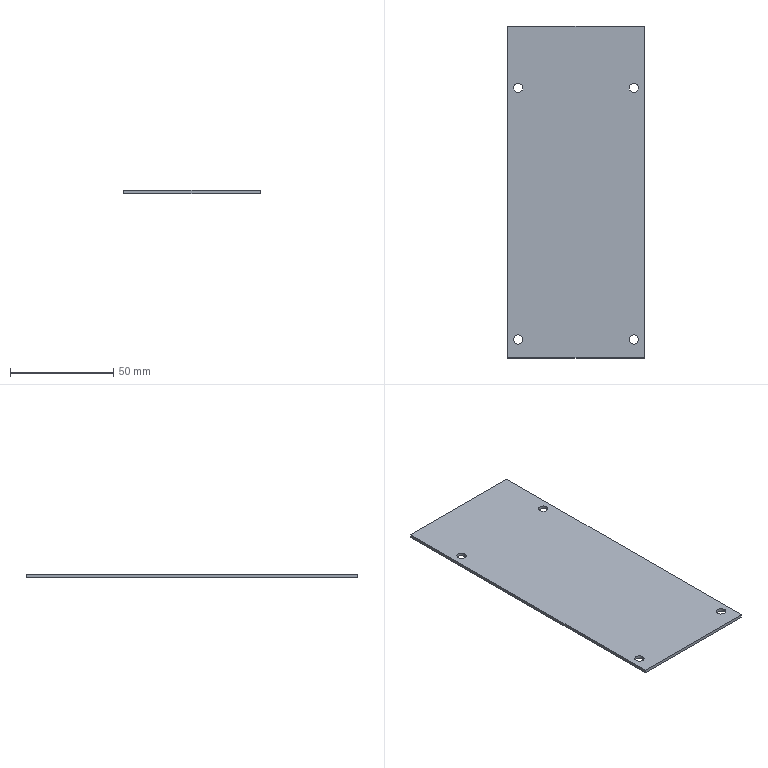Part | STEP file | 0245_219_Cover | 1 solid | 14 faces | box 66 x 161 x 1.5 mm | volume 15844 mm3 | cylinder 8 | plane 6 | commonest cylinder face diameters 4.5 x8
STEP:
#1=CARTESIAN_POINT('',(0.,0.,0.));
#2=DIRECTION('',(0.,0.,1.));
#3=DIRECTION('',(1.,0.,0.));
#4=AXIS2_PLACEMENT_3D('',#1,#2,#3);
#5=CARTESIAN_POINT('',(30.25,131.,0.));
#6=VERTEX_POINT('',#5);
#7=CARTESIAN_POINT('',(30.25,131.,1.5));
#8=VERTEX_POINT('',#7);
#9=CARTESIAN_POINT('',(30.25,131.,1.5));
#10=DIRECTION('',(0.,0.,1.));
#11=VECTOR('',#10,1.);
#12=LINE('',#9,#11);
#13=CARTESIAN_POINT('',(28.,131.,1.5));
#14=DIRECTION('',(0.,0.,1.));
#15=DIRECTION('',(1.,0.,0.));
#16=AXIS2_PLACEMENT_3D('',#13,#14,#15);
#17=CYLINDRICAL_SURFACE('',#16,2.25);
#18=CARTESIAN_POINT('',(6.283,0.));
#19=DIRECTION('',(0.,1.));
#20=VECTOR('',#19,1.);
#21=LINE('',#18,#20);
#22=(GEOMETRIC_REPRESENTATION_CONTEXT(2)PARAMETRIC_REPRESENTATION_CONTEXT()REPRESENTATION_CONTEXT('',''));
#23=DEFINITIONAL_REPRESENTATION('',(#21),#22);
#24=PCURVE('',#17,#23);
#25=CARTESIAN_POINT('',(28.,131.,1.5));
#26=DIRECTION('',(0.,0.,1.));
#27=DIRECTION('',(1.,0.,0.));
#28=AXIS2_PLACEMENT_3D('',#25,#26,#27);
#29=CYLINDRICAL_SURFACE('',#28,2.25);
#30=CARTESIAN_POINT('',(0.,0.));
#31=DIRECTION('',(0.,1.));
#32=VECTOR('',#31,1.);
#33=LINE('',#30,#32);
#34=(GEOMETRIC_REPRESENTATION_CONTEXT(2)PARAMETRIC_REPRESENTATION_CONTEXT()REPRESENTATION_CONTEXT('',''));
#35=DEFINITIONAL_REPRESENTATION('',(#33),#34);
#36=PCURVE('',#29,#35);
#37=SURFACE_CURVE('',#12,(#24,#36),.PCURVE_S1.);
#38=EDGE_CURVE('',#6,#8,#37,.T.);
#39=ORIENTED_EDGE('',*,*,#38,.T.);
#40=CARTESIAN_POINT('',(25.75,131.,1.5));
#41=VERTEX_POINT('',#40);
#42=CARTESIAN_POINT('',(28.,131.,1.5));
#43=DIRECTION('',(0.,0.,1.));
#44=DIRECTION('',(1.,0.,0.));
#45=AXIS2_PLACEMENT_3D('',#42,#43,#44);
#46=CIRCLE('',#45,2.25);
#47=CARTESIAN_POINT('',(0.,0.));
#48=DIRECTION('',(1.,0.));
#49=VECTOR('',#48,1.);
#50=LINE('',#47,#49);
#51=(GEOMETRIC_REPRESENTATION_CONTEXT(2)PARAMETRIC_REPRESENTATION_CONTEXT()REPRESENTATION_CONTEXT('',''));
#52=DEFINITIONAL_REPRESENTATION('',(#50),#51);
#53=PCURVE('',#17,#52);
#54=CARTESIAN_POINT('',(-33.,161.,1.5));
#55=DIRECTION('',(0.,0.,-1.));
#56=DIRECTION('',(-1.,0.,0.));
#57=AXIS2_PLACEMENT_3D('',#54,#55,#56);
#58=PLANE('',#57);
#59=CARTESIAN_POINT('',(-63.25,-30.));
#60=CARTESIAN_POINT('',(-63.25,-26.103));
#61=CARTESIAN_POINT('',(-59.875,-28.051));
#62=CARTESIAN_POINT('',(-56.5,-30.));
#63=CARTESIAN_POINT('',(-59.875,-31.949));
#64=CARTESIAN_POINT('',(-63.25,-33.897));
#65=CARTESIAN_POINT('',(-63.25,-30.));
#66=(BOUNDED_CURVE()B_SPLINE_CURVE(2,(#59,#60,#61,#62,#63,#64,#65),.UNSPECIFIED.,.T.,.F.)B_SPLINE_CURVE_WITH_KNOTS((1,2,2,2,2,1),(-2.094,0.,2.094,4.189,6.283,8.378),.UNSPECIFIED.)CURVE()GEOMETRIC_REPRESENTATION_ITEM()RATIONAL_B_SPLINE_CURVE((1.,0.5,1.,0.5,1.,0.5,1.))REPRESENTATION_ITEM(''));
#67=(GEOMETRIC_REPRESENTATION_CONTEXT(2)PARAMETRIC_REPRESENTATION_CONTEXT()REPRESENTATION_CONTEXT('',''));
#68=DEFINITIONAL_REPRESENTATION('',(#66),#67);
#69=PCURVE('',#58,#68);
#70=SURFACE_CURVE('',#46,(#53,#69),.PCURVE_S1.);
#71=EDGE_CURVE('',#41,#8,#70,.T.);
#72=ORIENTED_EDGE('',*,*,#71,.F.);
#73=CARTESIAN_POINT('',(25.75,131.,0.));
#74=VERTEX_POINT('',#73);
#75=CARTESIAN_POINT('',(25.75,131.,1.5));
#76=DIRECTION('',(0.,0.,1.));
#77=VECTOR('',#76,1.);
#78=LINE('',#75,#77);
#79=CARTESIAN_POINT('',(3.142,0.));
#80=DIRECTION('',(0.,1.));
#81=VECTOR('',#80,1.);
#82=LINE('',#79,#81);
#83=(GEOMETRIC_REPRESENTATION_CONTEXT(2)PARAMETRIC_REPRESENTATION_CONTEXT()REPRESENTATION_CONTEXT('',''));
#84=DEFINITIONAL_REPRESENTATION('',(#82),#83);
#85=PCURVE('',#17,#84);
#86=CARTESIAN_POINT('',(3.142,0.));
#87=DIRECTION('',(0.,1.));
#88=VECTOR('',#87,1.);
#89=LINE('',#86,#88);
#90=(GEOMETRIC_REPRESENTATION_CONTEXT(2)PARAMETRIC_REPRESENTATION_CONTEXT()REPRESENTATION_CONTEXT('',''));
#91=DEFINITIONAL_REPRESENTATION('',(#89),#90);
#92=PCURVE('',#29,#91);
#93=SURFACE_CURVE('',#78,(#85,#92),.PCURVE_S1.);
#94=EDGE_CURVE('',#74,#41,#93,.T.);
#95=ORIENTED_EDGE('',*,*,#94,.F.);
#96=CARTESIAN_POINT('',(28.,131.,0.));
#97=DIRECTION('',(0.,0.,1.));
#98=DIRECTION('',(1.,0.,0.));
#99=AXIS2_PLACEMENT_3D('',#96,#97,#98);
#100=CIRCLE('',#99,2.25);
#101=CARTESIAN_POINT('',(0.,-1.5));
#102=DIRECTION('',(1.,0.));
#103=VECTOR('',#102,1.);
#104=LINE('',#101,#103);
#105=(GEOMETRIC_REPRESENTATION_CONTEXT(2)PARAMETRIC_REPRESENTATION_CONTEXT()REPRESENTATION_CONTEXT('',''));
#106=DEFINITIONAL_REPRESENTATION('',(#104),#105);
#107=PCURVE('',#17,#106);
#108=CARTESIAN_POINT('',(-33.,161.,0.));
#109=DIRECTION('',(0.,0.,-1.));
#110=DIRECTION('',(-1.,0.,0.));
#111=AXIS2_PLACEMENT_3D('',#108,#109,#110);
#112=PLANE('',#111);
#113=CARTESIAN_POINT('',(-63.25,-30.));
#114=CARTESIAN_POINT('',(-63.25,-26.103));
#115=CARTESIAN_POINT('',(-59.875,-28.051));
#116=CARTESIAN_POINT('',(-56.5,-30.));
#117=CARTESIAN_POINT('',(-59.875,-31.949));
#118=CARTESIAN_POINT('',(-63.25,-33.897));
#119=CARTESIAN_POINT('',(-63.25,-30.));
#120=(BOUNDED_CURVE()B_SPLINE_CURVE(2,(#113,#114,#115,#116,#117,#118,#119),.UNSPECIFIED.,.T.,.F.)B_SPLINE_CURVE_WITH_KNOTS((1,2,2,2,2,1),(-2.094,0.,2.094,4.189,6.283,8.378),.UNSPECIFIED.)CURVE()GEOMETRIC_REPRESENTATION_ITEM()RATIONAL_B_SPLINE_CURVE((1.,0.5,1.,0.5,1.,0.5,1.))REPRESENTATION_ITEM(''));
#121=(GEOMETRIC_REPRESENTATION_CONTEXT(2)PARAMETRIC_REPRESENTATION_CONTEXT()REPRESENTATION_CONTEXT('',''));
#122=DEFINITIONAL_REPRESENTATION('',(#120),#121);
#123=PCURVE('',#112,#122);
#124=SURFACE_CURVE('',#100,(#107,#123),.PCURVE_S1.);
#125=EDGE_CURVE('',#74,#6,#124,.T.);
#126=ORIENTED_EDGE('',*,*,#125,.T.);
#127=EDGE_LOOP('',(#39,#72,#95,#126));
#128=FACE_BOUND('',#127,.F.);
#129=ADVANCED_FACE('',(#128),#17,.F.);
#130=CARTESIAN_POINT('',(-25.75,131.,0.));
#131=VERTEX_POINT('',#130);
#132=CARTESIAN_POINT('',(-25.75,131.,1.5));
#133=VERTEX_POINT('',#132);
#134=CARTESIAN_POINT('',(-25.75,131.,1.5));
#135=DIRECTION('',(0.,0.,1.));
#136=VECTOR('',#135,1.);
#137=LINE('',#134,#136);
#138=CARTESIAN_POINT('',(-28.,131.,1.5));
#139=DIRECTION('',(0.,0.,1.));
#140=DIRECTION('',(1.,0.,0.));
#141=AXIS2_PLACEMENT_3D('',#138,#139,#140);
#142=CYLINDRICAL_SURFACE('',#141,2.25);
#143=CARTESIAN_POINT('',(6.283,0.));
#144=DIRECTION('',(0.,1.));
#145=VECTOR('',#144,1.);
#146=LINE('',#143,#145);
#147=(GEOMETRIC_REPRESENTATION_CONTEXT(2)PARAMETRIC_REPRESENTATION_CONTEXT()REPRESENTATION_CONTEXT('',''));
#148=DEFINITIONAL_REPRESENTATION('',(#146),#147);
#149=PCURVE('',#142,#148);
#150=CARTESIAN_POINT('',(-28.,131.,1.5));
#151=DIRECTION('',(0.,0.,1.));
#152=DIRECTION('',(1.,0.,0.));
#153=AXIS2_PLACEMENT_3D('',#150,#151,#152);
#154=CYLINDRICAL_SURFACE('',#153,2.25);
#155=CARTESIAN_POINT('',(0.,0.));
#156=DIRECTION('',(0.,1.));
#157=VECTOR('',#156,1.);
#158=LINE('',#155,#157);
#159=(GEOMETRIC_REPRESENTATION_CONTEXT(2)PARAMETRIC_REPRESENTATION_CONTEXT()REPRESENTATION_CONTEXT('',''));
#160=DEFINITIONAL_REPRESENTATION('',(#158),#159);
#161=PCURVE('',#154,#160);
#162=SURFACE_CURVE('',#137,(#149,#161),.PCURVE_S1.);
#163=EDGE_CURVE('',#131,#133,#162,.T.);
#164=ORIENTED_EDGE('',*,*,#163,.T.);
#165=CARTESIAN_POINT('',(-30.25,131.,1.5));
#166=VERTEX_POINT('',#165);
#167=CARTESIAN_POINT('',(-28.,131.,1.5));
#168=DIRECTION('',(0.,0.,1.));
#169=DIRECTION('',(1.,0.,0.));
#170=AXIS2_PLACEMENT_3D('',#167,#168,#169);
#171=CIRCLE('',#170,2.25);
#172=CARTESIAN_POINT('',(0.,0.));
#173=DIRECTION('',(1.,0.));
#174=VECTOR('',#173,1.);
#175=LINE('',#172,#174);
#176=(GEOMETRIC_REPRESENTATION_CONTEXT(2)PARAMETRIC_REPRESENTATION_CONTEXT()REPRESENTATION_CONTEXT('',''));
#177=DEFINITIONAL_REPRESENTATION('',(#175),#176);
#178=PCURVE('',#142,#177);
#179=CARTESIAN_POINT('',(-7.25,-30.));
#180=CARTESIAN_POINT('',(-7.25,-26.103));
#181=CARTESIAN_POINT('',(-3.875,-28.051));
#182=CARTESIAN_POINT('',(-0.5,-30.));
#183=CARTESIAN_POINT('',(-3.875,-31.949));
#184=CARTESIAN_POINT('',(-7.25,-33.897));
#185=CARTESIAN_POINT('',(-7.25,-30.));
#186=(BOUNDED_CURVE()B_SPLINE_CURVE(2,(#179,#180,#181,#182,#183,#184,#185),.UNSPECIFIED.,.T.,.F.)B_SPLINE_CURVE_WITH_KNOTS((1,2,2,2,2,1),(-2.094,0.,2.094,4.189,6.283,8.378),.UNSPECIFIED.)CURVE()GEOMETRIC_REPRESENTATION_ITEM()RATIONAL_B_SPLINE_CURVE((1.,0.5,1.,0.5,1.,0.5,1.))REPRESENTATION_ITEM(''));
#187=(GEOMETRIC_REPRESENTATION_CONTEXT(2)PARAMETRIC_REPRESENTATION_CONTEXT()REPRESENTATION_CONTEXT('',''));
#188=DEFINITIONAL_REPRESENTATION('',(#186),#187);
#189=PCURVE('',#58,#188);
#190=SURFACE_CURVE('',#171,(#178,#189),.PCURVE_S1.);
#191=EDGE_CURVE('',#166,#133,#190,.T.);
#192=ORIENTED_EDGE('',*,*,#191,.F.);
#193=CARTESIAN_POINT('',(-30.25,131.,0.));
#194=VERTEX_POINT('',#193);
#195=CARTESIAN_POINT('',(-30.25,131.,1.5));
#196=DIRECTION('',(0.,0.,1.));
#197=VECTOR('',#196,1.);
#198=LINE('',#195,#197);
#199=CARTESIAN_POINT('',(3.142,0.));
#200=DIRECTION('',(0.,1.));
#201=VECTOR('',#200,1.);
#202=LINE('',#199,#201);
#203=(GEOMETRIC_REPRESENTATION_CONTEXT(2)PARAMETRIC_REPRESENTATION_CONTEXT()REPRESENTATION_CONTEXT('',''));
#204=DEFINITIONAL_REPRESENTATION('',(#202),#203);
#205=PCURVE('',#142,#204);
#206=CARTESIAN_POINT('',(3.142,0.));
#207=DIRECTION('',(0.,1.));
#208=VECTOR('',#207,1.);
#209=LINE('',#206,#208);
#210=(GEOMETRIC_REPRESENTATION_CONTEXT(2)PARAMETRIC_REPRESENTATION_CONTEXT()REPRESENTATION_CONTEXT('',''));
#211=DEFINITIONAL_REPRESENTATION('',(#209),#210);
#212=PCURVE('',#154,#211);
#213=SURFACE_CURVE('',#198,(#205,#212),.PCURVE_S1.);
#214=EDGE_CURVE('',#194,#166,#213,.T.);
#215=ORIENTED_EDGE('',*,*,#214,.F.);
#216=CARTESIAN_POINT('',(-28.,131.,0.));
#217=DIRECTION('',(0.,0.,1.));
#218=DIRECTION('',(1.,0.,0.));
#219=AXIS2_PLACEMENT_3D('',#216,#217,#218);
#220=CIRCLE('',#219,2.25);
#221=CARTESIAN_POINT('',(0.,-1.5));
#222=DIRECTION('',(1.,0.));
#223=VECTOR('',#222,1.);
#224=LINE('',#221,#223);
#225=(GEOMETRIC_REPRESENTATION_CONTEXT(2)PARAMETRIC_REPRESENTATION_CONTEXT()REPRESENTATION_CONTEXT('',''));
#226=DEFINITIONAL_REPRESENTATION('',(#224),#225);
#227=PCURVE('',#142,#226);
#228=CARTESIAN_POINT('',(-7.25,-30.));
#229=CARTESIAN_POINT('',(-7.25,-26.103));
#230=CARTESIAN_POINT('',(-3.875,-28.051));
#231=CARTESIAN_POINT('',(-0.5,-30.));
#232=CARTESIAN_POINT('',(-3.875,-31.949));
#233=CARTESIAN_POINT('',(-7.25,-33.897));
#234=CARTESIAN_POINT('',(-7.25,-30.));
#235=(BOUNDED_CURVE()B_SPLINE_CURVE(2,(#228,#229,#230,#231,#232,#233,#234),.UNSPECIFIED.,.T.,.F.)B_SPLINE_CURVE_WITH_KNOTS((1,2,2,2,2,1),(-2.094,0.,2.094,4.189,6.283,8.378),.UNSPECIFIED.)CURVE()GEOMETRIC_REPRESENTATION_ITEM()RATIONAL_B_SPLINE_CURVE((1.,0.5,1.,0.5,1.,0.5,1.))REPRESENTATION_ITEM(''));
#236=(GEOMETRIC_REPRESENTATION_CONTEXT(2)PARAMETRIC_REPRESENTATION_CONTEXT()REPRESENTATION_CONTEXT('',''));
#237=DEFINITIONAL_REPRESENTATION('',(#235),#236);
#238=PCURVE('',#112,#237);
#239=SURFACE_CURVE('',#220,(#227,#238),.PCURVE_S1.);
#240=EDGE_CURVE('',#194,#131,#239,.T.);
#241=ORIENTED_EDGE('',*,*,#240,.T.);
#242=EDGE_LOOP('',(#164,#192,#215,#241));
#243=FACE_BOUND('',#242,.F.);
#244=ADVANCED_FACE('',(#243),#142,.F.);
#245=CARTESIAN_POINT('',(30.25,9.,0.));
#246=VERTEX_POINT('',#245);
#247=CARTESIAN_POINT('',(30.25,9.,1.5));
#248=VERTEX_POINT('',#247);
#249=CARTESIAN_POINT('',(30.25,9.,1.5));
#250=DIRECTION('',(0.,0.,1.));
#251=VECTOR('',#250,1.);
#252=LINE('',#249,#251);
#253=CARTESIAN_POINT('',(28.,9.,1.5));
#254=DIRECTION('',(0.,0.,1.));
#255=DIRECTION('',(1.,0.,0.));
#256=AXIS2_PLACEMENT_3D('',#253,#254,#255);
#257=CYLINDRICAL_SURFACE('',#256,2.25);
#258=CARTESIAN_POINT('',(6.283,0.));
#259=DIRECTION('',(0.,1.));
#260=VECTOR('',#259,1.);
#261=LINE('',#258,#260);
#262=(GEOMETRIC_REPRESENTATION_CONTEXT(2)PARAMETRIC_REPRESENTATION_CONTEXT()REPRESENTATION_CONTEXT('',''));
#263=DEFINITIONAL_REPRESENTATION('',(#261),#262);
#264=PCURVE('',#257,#263);
#265=CARTESIAN_POINT('',(28.,9.,1.5));
#266=DIRECTION('',(0.,0.,1.));
#267=DIRECTION('',(1.,0.,0.));
#268=AXIS2_PLACEMENT_3D('',#265,#266,#267);
#269=CYLINDRICAL_SURFACE('',#268,2.25);
#270=CARTESIAN_POINT('',(0.,0.));
#271=DIRECTION('',(0.,1.));
#272=VECTOR('',#271,1.);
#273=LINE('',#270,#272);
#274=(GEOMETRIC_REPRESENTATION_CONTEXT(2)PARAMETRIC_REPRESENTATION_CONTEXT()REPRESENTATION_CONTEXT('',''));
#275=DEFINITIONAL_REPRESENTATION('',(#273),#274);
#276=PCURVE('',#269,#275);
#277=SURFACE_CURVE('',#252,(#264,#276),.PCURVE_S1.);
#278=EDGE_CURVE('',#246,#248,#277,.T.);
#279=ORIENTED_EDGE('',*,*,#278,.T.);
#280=CARTESIAN_POINT('',(25.75,9.,1.5));
#281=VERTEX_POINT('',#280);
#282=CARTESIAN_POINT('',(28.,9.,1.5));
#283=DIRECTION('',(0.,0.,1.));
#284=DIRECTION('',(1.,0.,0.));
#285=AXIS2_PLACEMENT_3D('',#282,#283,#284);
#286=CIRCLE('',#285,2.25);
#287=CARTESIAN_POINT('',(0.,0.));
#288=DIRECTION('',(1.,0.));
#289=VECTOR('',#288,1.);
#290=LINE('',#287,#289);
#291=(GEOMETRIC_REPRESENTATION_CONTEXT(2)PARAMETRIC_REPRESENTATION_CONTEXT()REPRESENTATION_CONTEXT('',''));
#292=DEFINITIONAL_REPRESENTATION('',(#290),#291);
#293=PCURVE('',#257,#292);
#294=CARTESIAN_POINT('',(-63.25,-152.));
#295=CARTESIAN_POINT('',(-63.25,-148.103));
#296=CARTESIAN_POINT('',(-59.875,-150.051));
#297=CARTESIAN_POINT('',(-56.5,-152.));
#298=CARTESIAN_POINT('',(-59.875,-153.949));
#299=CARTESIAN_POINT('',(-63.25,-155.897));
#300=CARTESIAN_POINT('',(-63.25,-152.));
#301=(BOUNDED_CURVE()B_SPLINE_CURVE(2,(#294,#295,#296,#297,#298,#299,#300),.UNSPECIFIED.,.T.,.F.)B_SPLINE_CURVE_WITH_KNOTS((1,2,2,2,2,1),(-2.094,0.,2.094,4.189,6.283,8.378),.UNSPECIFIED.)CURVE()GEOMETRIC_REPRESENTATION_ITEM()RATIONAL_B_SPLINE_CURVE((1.,0.5,1.,0.5,1.,0.5,1.))REPRESENTATION_ITEM(''));
#302=(GEOMETRIC_REPRESENTATION_CONTEXT(2)PARAMETRIC_REPRESENTATION_CONTEXT()REPRESENTATION_CONTEXT('',''));
#303=DEFINITIONAL_REPRESENTATION('',(#301),#302);
#304=PCURVE('',#58,#303);
#305=SURFACE_CURVE('',#286,(#293,#304),.PCURVE_S1.);
#306=EDGE_CURVE('',#281,#248,#305,.T.);
#307=ORIENTED_EDGE('',*,*,#306,.F.);
#308=CARTESIAN_POINT('',(25.75,9.,0.));
#309=VERTEX_POINT('',#308);
#310=CARTESIAN_POINT('',(25.75,9.,1.5));
#311=DIRECTION('',(0.,0.,1.));
#312=VECTOR('',#311,1.);
#313=LINE('',#310,#312);
#314=CARTESIAN_POINT('',(3.142,0.));
#315=DIRECTION('',(0.,1.));
#316=VECTOR('',#315,1.);
#317=LINE('',#314,#316);
#318=(GEOMETRIC_REPRESENTATION_CONTEXT(2)PARAMETRIC_REPRESENTATION_CONTEXT()REPRESENTATION_CONTEXT('',''));
#319=DEFINITIONAL_REPRESENTATION('',(#317),#318);
#320=PCURVE('',#257,#319);
#321=CARTESIAN_POINT('',(3.142,0.));
#322=DIRECTION('',(0.,1.));
#323=VECTOR('',#322,1.);
#324=LINE('',#321,#323);
#325=(GEOMETRIC_REPRESENTATION_CONTEXT(2)PARAMETRIC_REPRESENTATION_CONTEXT()REPRESENTATION_CONTEXT('',''));
#326=DEFINITIONAL_REPRESENTATION('',(#324),#325);
#327=PCURVE('',#269,#326);
#328=SURFACE_CURVE('',#313,(#320,#327),.PCURVE_S1.);
#329=EDGE_CURVE('',#309,#281,#328,.T.);
#330=ORIENTED_EDGE('',*,*,#329,.F.);
#331=CARTESIAN_POINT('',(28.,9.,0.));
#332=DIRECTION('',(0.,0.,1.));
#333=DIRECTION('',(1.,0.,0.));
#334=AXIS2_PLACEMENT_3D('',#331,#332,#333);
#335=CIRCLE('',#334,2.25);
#336=CARTESIAN_POINT('',(0.,-1.5));
#337=DIRECTION('',(1.,0.));
#338=VECTOR('',#337,1.);
#339=LINE('',#336,#338);
#340=(GEOMETRIC_REPRESENTATION_CONTEXT(2)PARAMETRIC_REPRESENTATION_CONTEXT()REPRESENTATION_CONTEXT('',''));
#341=DEFINITIONAL_REPRESENTATION('',(#339),#340);
#342=PCURVE('',#257,#341);
#343=CARTESIAN_POINT('',(-63.25,-152.));
#344=CARTESIAN_POINT('',(-63.25,-148.103));
#345=CARTESIAN_POINT('',(-59.875,-150.051));
#346=CARTESIAN_POINT('',(-56.5,-152.));
#347=CARTESIAN_POINT('',(-59.875,-153.949));
#348=CARTESIAN_POINT('',(-63.25,-155.897));
#349=CARTESIAN_POINT('',(-63.25,-152.));
#350=(BOUNDED_CURVE()B_SPLINE_CURVE(2,(#343,#344,#345,#346,#347,#348,#349),.UNSPECIFIED.,.T.,.F.)B_SPLINE_CURVE_WITH_KNOTS((1,2,2,2,2,1),(-2.094,0.,2.094,4.189,6.283,8.378),.UNSPECIFIED.)CURVE()GEOMETRIC_REPRESENTATION_ITEM()RATIONAL_B_SPLINE_CURVE((1.,0.5,1.,0.5,1.,0.5,1.))REPRESENTATION_ITEM(''));
#351=(GEOMETRIC_REPRESENTATION_CONTEXT(2)PARAMETRIC_REPRESENTATION_CONTEXT()REPRESENTATION_CONTEXT('',''));
#352=DEFINITIONAL_REPRESENTATION('',(#350),#351);
#353=PCURVE('',#112,#352);
#354=SURFACE_CURVE('',#335,(#342,#353),.PCURVE_S1.);
#355=EDGE_CURVE('',#309,#246,#354,.T.);
#356=ORIENTED_EDGE('',*,*,#355,.T.);
#357=EDGE_LOOP('',(#279,#307,#330,#356));
#358=FACE_BOUND('',#357,.F.);
#359=ADVANCED_FACE('',(#358),#257,.F.);
#360=CARTESIAN_POINT('',(-25.75,9.,0.));
#361=VERTEX_POINT('',#360);
#362=CARTESIAN_POINT('',(-25.75,9.,1.5));
#363=VERTEX_POINT('',#362);
#364=CARTESIAN_POINT('',(-25.75,9.,1.5));
#365=DIRECTION('',(0.,0.,1.));
#366=VECTOR('',#365,1.);
#367=LINE('',#364,#366);
#368=CARTESIAN_POINT('',(-28.,9.,1.5));
#369=DIRECTION('',(0.,0.,1.));
#370=DIRECTION('',(1.,0.,0.));
#371=AXIS2_PLACEMENT_3D('',#368,#369,#370);
#372=CYLINDRICAL_SURFACE('',#371,2.25);
#373=CARTESIAN_POINT('',(6.283,0.));
#374=DIRECTION('',(0.,1.));
#375=VECTOR('',#374,1.);
#376=LINE('',#373,#375);
#377=(GEOMETRIC_REPRESENTATION_CONTEXT(2)PARAMETRIC_REPRESENTATION_CONTEXT()REPRESENTATION_CONTEXT('',''));
#378=DEFINITIONAL_REPRESENTATION('',(#376),#377);
#379=PCURVE('',#372,#378);
#380=CARTESIAN_POINT('',(-28.,9.,1.5));
#381=DIRECTION('',(0.,0.,1.));
#382=DIRECTION('',(1.,0.,0.));
#383=AXIS2_PLACEMENT_3D('',#380,#381,#382);
#384=CYLINDRICAL_SURFACE('',#383,2.25);
#385=CARTESIAN_POINT('',(0.,0.));
#386=DIRECTION('',(0.,1.));
#387=VECTOR('',#386,1.);
#388=LINE('',#385,#387);
#389=(GEOMETRIC_REPRESENTATION_CONTEXT(2)PARAMETRIC_REPRESENTATION_CONTEXT()REPRESENTATION_CONTEXT('',''));
#390=DEFINITIONAL_REPRESENTATION('',(#388),#389);
#391=PCURVE('',#384,#390);
#392=SURFACE_CURVE('',#367,(#379,#391),.PCURVE_S1.);
#393=EDGE_CURVE('',#361,#363,#392,.T.);
#394=ORIENTED_EDGE('',*,*,#393,.T.);
#395=CARTESIAN_POINT('',(-30.25,9.,1.5));
#396=VERTEX_POINT('',#395);
#397=CARTESIAN_POINT('',(-28.,9.,1.5));
#398=DIRECTION('',(0.,0.,1.));
#399=DIRECTION('',(1.,0.,0.));
#400=AXIS2_PLACEMENT_3D('',#397,#398,#399);
#401=CIRCLE('',#400,2.25);
#402=CARTESIAN_POINT('',(0.,0.));
#403=DIRECTION('',(1.,0.));
#404=VECTOR('',#403,1.);
#405=LINE('',#402,#404);
#406=(GEOMETRIC_REPRESENTATION_CONTEXT(2)PARAMETRIC_REPRESENTATION_CONTEXT()REPRESENTATION_CONTEXT('',''));
#407=DEFINITIONAL_REPRESENTATION('',(#405),#406);
#408=PCURVE('',#372,#407);
#409=CARTESIAN_POINT('',(-7.25,-152.));
#410=CARTESIAN_POINT('',(-7.25,-148.103));
#411=CARTESIAN_POINT('',(-3.875,-150.051));
#412=CARTESIAN_POINT('',(-0.5,-152.));
#413=CARTESIAN_POINT('',(-3.875,-153.949));
#414=CARTESIAN_POINT('',(-7.25,-155.897));
#415=CARTESIAN_POINT('',(-7.25,-152.));
#416=(BOUNDED_CURVE()B_SPLINE_CURVE(2,(#409,#410,#411,#412,#413,#414,#415),.UNSPECIFIED.,.T.,.F.)B_SPLINE_CURVE_WITH_KNOTS((1,2,2,2,2,1),(-2.094,0.,2.094,4.189,6.283,8.378),.UNSPECIFIED.)CURVE()GEOMETRIC_REPRESENTATION_ITEM()RATIONAL_B_SPLINE_CURVE((1.,0.5,1.,0.5,1.,0.5,1.))REPRESENTATION_ITEM(''));
#417=(GEOMETRIC_REPRESENTATION_CONTEXT(2)PARAMETRIC_REPRESENTATION_CONTEXT()REPRESENTATION_CONTEXT('',''));
#418=DEFINITIONAL_REPRESENTATION('',(#416),#417);
#419=PCURVE('',#58,#418);
#420=SURFACE_CURVE('',#401,(#408,#419),.PCURVE_S1.);
#421=EDGE_CURVE('',#396,#363,#420,.T.);
#422=ORIENTED_EDGE('',*,*,#421,.F.);
#423=CARTESIAN_POINT('',(-30.25,9.,0.));
#424=VERTEX_POINT('',#423);
#425=CARTESIAN_POINT('',(-30.25,9.,1.5));
#426=DIRECTION('',(0.,0.,1.));
#427=VECTOR('',#426,1.);
#428=LINE('',#425,#427);
#429=CARTESIAN_POINT('',(3.142,0.));
#430=DIRECTION('',(0.,1.));
#431=VECTOR('',#430,1.);
#432=LINE('',#429,#431);
#433=(GEOMETRIC_REPRESENTATION_CONTEXT(2)PARAMETRIC_REPRESENTATION_CONTEXT()REPRESENTATION_CONTEXT('',''));
#434=DEFINITIONAL_REPRESENTATION('',(#432),#433);
#435=PCURVE('',#372,#434);
#436=CARTESIAN_POINT('',(3.142,0.));
#437=DIRECTION('',(0.,1.));
#438=VECTOR('',#437,1.);
#439=LINE('',#436,#438);
#440=(GEOMETRIC_REPRESENTATION_CONTEXT(2)PARAMETRIC_REPRESENTATION_CONTEXT()REPRESENTATION_CONTEXT('',''));
#441=DEFINITIONAL_REPRESENTATION('',(#439),#440);
#442=PCURVE('',#384,#441);
#443=SURFACE_CURVE('',#428,(#435,#442),.PCURVE_S1.);
#444=EDGE_CURVE('',#424,#396,#443,.T.);
#445=ORIENTED_EDGE('',*,*,#444,.F.);
#446=CARTESIAN_POINT('',(-28.,9.,0.));
#447=DIRECTION('',(0.,0.,1.));
#448=DIRECTION('',(1.,0.,0.));
#449=AXIS2_PLACEMENT_3D('',#446,#447,#448);
#450=CIRCLE('',#449,2.25);
#451=CARTESIAN_POINT('',(0.,-1.5));
#452=DIRECTION('',(1.,0.));
#453=VECTOR('',#452,1.);
#454=LINE('',#451,#453);
#455=(GEOMETRIC_REPRESENTATION_CONTEXT(2)PARAMETRIC_REPRESENTATION_CONTEXT()REPRESENTATION_CONTEXT('',''));
#456=DEFINITIONAL_REPRESENTATION('',(#454),#455);
#457=PCURVE('',#372,#456);
#458=CARTESIAN_POINT('',(-7.25,-152.));
#459=CARTESIAN_POINT('',(-7.25,-148.103));
#460=CARTESIAN_POINT('',(-3.875,-150.051));
#461=CARTESIAN_POINT('',(-0.5,-152.));
#462=CARTESIAN_POINT('',(-3.875,-153.949));
#463=CARTESIAN_POINT('',(-7.25,-155.897));
#464=CARTESIAN_POINT('',(-7.25,-152.));
#465=(BOUNDED_CURVE()B_SPLINE_CURVE(2,(#458,#459,#460,#461,#462,#463,#464),.UNSPECIFIED.,.T.,.F.)B_SPLINE_CURVE_WITH_KNOTS((1,2,2,2,2,1),(-2.094,0.,2.094,4.189,6.283,8.378),.UNSPECIFIED.)CURVE()GEOMETRIC_REPRESENTATION_ITEM()RATIONAL_B_SPLINE_CURVE((1.,0.5,1.,0.5,1.,0.5,1.))REPRESENTATION_ITEM(''));
#466=(GEOMETRIC_REPRESENTATION_CONTEXT(2)PARAMETRIC_REPRESENTATION_CONTEXT()REPRESENTATION_CONTEXT('',''));
#467=DEFINITIONAL_REPRESENTATION('',(#465),#466);
#468=PCURVE('',#112,#467);
#469=SURFACE_CURVE('',#450,(#457,#468),.PCURVE_S1.);
#470=EDGE_CURVE('',#424,#361,#469,.T.);
#471=ORIENTED_EDGE('',*,*,#470,.T.);
#472=EDGE_LOOP('',(#394,#422,#445,#471));
#473=FACE_BOUND('',#472,.F.);
#474=ADVANCED_FACE('',(#473),#372,.F.);
#475=CARTESIAN_POINT('',(-33.,161.,0.));
#476=VERTEX_POINT('',#475);
#477=CARTESIAN_POINT('',(-33.,0.,0.));
#478=VERTEX_POINT('',#477);
#479=CARTESIAN_POINT('',(-33.,0.,0.));
#480=DIRECTION('',(0.,-1.,0.));
#481=VECTOR('',#480,1.);
#482=LINE('',#479,#481);
#483=CARTESIAN_POINT('',(-33.,0.,1.5));
#484=DIRECTION('',(1.,0.,0.));
#485=DIRECTION('',(0.,0.,-1.));
#486=AXIS2_PLACEMENT_3D('',#483,#484,#485);
#487=PLANE('',#486);
#488=CARTESIAN_POINT('',(1.5,0.));
#489=DIRECTION('',(0.,-1.));
#490=VECTOR('',#489,1.);
#491=LINE('',#488,#490);
#492=(GEOMETRIC_REPRESENTATION_CONTEXT(2)PARAMETRIC_REPRESENTATION_CONTEXT()REPRESENTATION_CONTEXT('',''));
#493=DEFINITIONAL_REPRESENTATION('',(#491),#492);
#494=PCURVE('',#487,#493);
#495=CARTESIAN_POINT('',(0.,-161.));
#496=DIRECTION('',(0.,-1.));
#497=VECTOR('',#496,1.);
#498=LINE('',#495,#497);
#499=(GEOMETRIC_REPRESENTATION_CONTEXT(2)PARAMETRIC_REPRESENTATION_CONTEXT()REPRESENTATION_CONTEXT('',''));
#500=DEFINITIONAL_REPRESENTATION('',(#498),#499);
#501=PCURVE('',#112,#500);
#502=SURFACE_CURVE('',#482,(#494,#501),.PCURVE_S1.);
#503=EDGE_CURVE('',#476,#478,#502,.T.);
#504=ORIENTED_EDGE('',*,*,#503,.T.);
#505=CARTESIAN_POINT('',(-33.,0.,1.5));
#506=VERTEX_POINT('',#505);
#507=CARTESIAN_POINT('',(-33.,0.,1.5));
#508=DIRECTION('',(0.,0.,-1.));
#509=VECTOR('',#508,1.);
#510=LINE('',#507,#509);
#511=CARTESIAN_POINT('',(0.,0.));
#512=DIRECTION('',(1.,0.));
#513=VECTOR('',#512,1.);
#514=LINE('',#511,#513);
#515=(GEOMETRIC_REPRESENTATION_CONTEXT(2)PARAMETRIC_REPRESENTATION_CONTEXT()REPRESENTATION_CONTEXT('',''));
#516=DEFINITIONAL_REPRESENTATION('',(#514),#515);
#517=PCURVE('',#487,#516);
#518=CARTESIAN_POINT('',(-33.,0.,1.5));
#519=DIRECTION('',(0.,1.,0.));
#520=DIRECTION('',(0.,0.,1.));
#521=AXIS2_PLACEMENT_3D('',#518,#519,#520);
#522=PLANE('',#521);
#523=CARTESIAN_POINT('',(0.,0.));
#524=DIRECTION('',(-1.,0.));
#525=VECTOR('',#524,1.);
#526=LINE('',#523,#525);
#527=(GEOMETRIC_REPRESENTATION_CONTEXT(2)PARAMETRIC_REPRESENTATION_CONTEXT()REPRESENTATION_CONTEXT('',''));
#528=DEFINITIONAL_REPRESENTATION('',(#526),#527);
#529=PCURVE('',#522,#528);
#530=SURFACE_CURVE('',#510,(#517,#529),.PCURVE_S1.);
#531=EDGE_CURVE('',#506,#478,#530,.T.);
#532=ORIENTED_EDGE('',*,*,#531,.F.);
#533=CARTESIAN_POINT('',(-33.,161.,1.5));
#534=VERTEX_POINT('',#533);
#535=CARTESIAN_POINT('',(-33.,0.,1.5));
#536=DIRECTION('',(0.,-1.,0.));
#537=VECTOR('',#536,1.);
#538=LINE('',#535,#537);
#539=CARTESIAN_POINT('',(0.,0.));
#540=DIRECTION('',(0.,-1.));
#541=VECTOR('',#540,1.);
#542=LINE('',#539,#541);
#543=(GEOMETRIC_REPRESENTATION_CONTEXT(2)PARAMETRIC_REPRESENTATION_CONTEXT()REPRESENTATION_CONTEXT('',''));
#544=DEFINITIONAL_REPRESENTATION('',(#542),#543);
#545=PCURVE('',#487,#544);
#546=CARTESIAN_POINT('',(0.,-161.));
#547=DIRECTION('',(0.,-1.));
#548=VECTOR('',#547,1.);
#549=LINE('',#546,#548);
#550=(GEOMETRIC_REPRESENTATION_CONTEXT(2)PARAMETRIC_REPRESENTATION_CONTEXT()REPRESENTATION_CONTEXT('',''));
#551=DEFINITIONAL_REPRESENTATION('',(#549),#550);
#552=PCURVE('',#58,#551);
#553=SURFACE_CURVE('',#538,(#545,#552),.PCURVE_S1.);
#554=EDGE_CURVE('',#534,#506,#553,.T.);
#555=ORIENTED_EDGE('',*,*,#554,.F.);
#556=CARTESIAN_POINT('',(-33.,161.,1.5));
#557=DIRECTION('',(0.,0.,-1.));
#558=VECTOR('',#557,1.);
#559=LINE('',#556,#558);
#560=CARTESIAN_POINT('',(0.,161.));
#561=DIRECTION('',(1.,0.));
#562=VECTOR('',#561,1.);
#563=LINE('',#560,#562);
#564=(GEOMETRIC_REPRESENTATION_CONTEXT(2)PARAMETRIC_REPRESENTATION_CONTEXT()REPRESENTATION_CONTEXT('',''));
#565=DEFINITIONAL_REPRESENTATION('',(#563),#564);
#566=PCURVE('',#487,#565);
#567=CARTESIAN_POINT('',(-33.,161.,1.5));
#568=DIRECTION('',(0.,-1.,0.));
#569=DIRECTION('',(0.,0.,-1.));
#570=AXIS2_PLACEMENT_3D('',#567,#568,#569);
#571=PLANE('',#570);
#572=CARTESIAN_POINT('',(0.,0.));
#573=DIRECTION('',(1.,0.));
#574=VECTOR('',#573,1.);
#575=LINE('',#572,#574);
#576=(GEOMETRIC_REPRESENTATION_CONTEXT(2)PARAMETRIC_REPRESENTATION_CONTEXT()REPRESENTATION_CONTEXT('',''));
#577=DEFINITIONAL_REPRESENTATION('',(#575),#576);
#578=PCURVE('',#571,#577);
#579=SURFACE_CURVE('',#559,(#566,#578),.PCURVE_S1.);
#580=EDGE_CURVE('',#534,#476,#579,.T.);
#581=ORIENTED_EDGE('',*,*,#580,.T.);
#582=EDGE_LOOP('',(#504,#532,#555,#581));
#583=FACE_BOUND('',#582,.T.);
#584=ADVANCED_FACE('',(#583),#487,.F.);
#585=CARTESIAN_POINT('',(33.,0.,0.));
#586=VERTEX_POINT('',#585);
#587=CARTESIAN_POINT('',(-33.,0.,0.));
#588=DIRECTION('',(1.,0.,0.));
#589=VECTOR('',#588,1.);
#590=LINE('',#587,#589);
#591=CARTESIAN_POINT('',(-1.5,0.));
#592=DIRECTION('',(0.,1.));
#593=VECTOR('',#592,1.);
#594=LINE('',#591,#593);
#595=(GEOMETRIC_REPRESENTATION_CONTEXT(2)PARAMETRIC_REPRESENTATION_CONTEXT()REPRESENTATION_CONTEXT('',''));
#596=DEFINITIONAL_REPRESENTATION('',(#594),#595);
#597=PCURVE('',#522,#596);
#598=CARTESIAN_POINT('',(0.,-161.));
#599=DIRECTION('',(-1.,0.));
#600=VECTOR('',#599,1.);
#601=LINE('',#598,#600);
#602=(GEOMETRIC_REPRESENTATION_CONTEXT(2)PARAMETRIC_REPRESENTATION_CONTEXT()REPRESENTATION_CONTEXT('',''));
#603=DEFINITIONAL_REPRESENTATION('',(#601),#602);
#604=PCURVE('',#112,#603);
#605=SURFACE_CURVE('',#590,(#597,#604),.PCURVE_S1.);
#606=EDGE_CURVE('',#478,#586,#605,.T.);
#607=ORIENTED_EDGE('',*,*,#606,.T.);
#608=CARTESIAN_POINT('',(33.,0.,1.5));
#609=VERTEX_POINT('',#608);
#610=CARTESIAN_POINT('',(33.,0.,1.5));
#611=DIRECTION('',(0.,0.,-1.));
#612=VECTOR('',#611,1.);
#613=LINE('',#610,#612);
#614=CARTESIAN_POINT('',(0.,66.));
#615=DIRECTION('',(-1.,0.));
#616=VECTOR('',#615,1.);
#617=LINE('',#614,#616);
#618=(GEOMETRIC_REPRESENTATION_CONTEXT(2)PARAMETRIC_REPRESENTATION_CONTEXT()REPRESENTATION_CONTEXT('',''));
#619=DEFINITIONAL_REPRESENTATION('',(#617),#618);
#620=PCURVE('',#522,#619);
#621=CARTESIAN_POINT('',(33.,0.,1.5));
#622=DIRECTION('',(-1.,0.,0.));
#623=DIRECTION('',(0.,0.,1.));
#624=AXIS2_PLACEMENT_3D('',#621,#622,#623);
#625=PLANE('',#624);
#626=CARTESIAN_POINT('',(0.,0.));
#627=DIRECTION('',(-1.,0.));
#628=VECTOR('',#627,1.);
#629=LINE('',#626,#628);
#630=(GEOMETRIC_REPRESENTATION_CONTEXT(2)PARAMETRIC_REPRESENTATION_CONTEXT()REPRESENTATION_CONTEXT('',''));
#631=DEFINITIONAL_REPRESENTATION('',(#629),#630);
#632=PCURVE('',#625,#631);
#633=SURFACE_CURVE('',#613,(#620,#632),.PCURVE_S1.);
#634=EDGE_CURVE('',#609,#586,#633,.T.);
#635=ORIENTED_EDGE('',*,*,#634,.F.);
#636=CARTESIAN_POINT('',(-33.,0.,1.5));
#637=DIRECTION('',(1.,0.,0.));
#638=VECTOR('',#637,1.);
#639=LINE('',#636,#638);
#640=CARTESIAN_POINT('',(0.,0.));
#641=DIRECTION('',(0.,1.));
#642=VECTOR('',#641,1.);
#643=LINE('',#640,#642);
#644=(GEOMETRIC_REPRESENTATION_CONTEXT(2)PARAMETRIC_REPRESENTATION_CONTEXT()REPRESENTATION_CONTEXT('',''));
#645=DEFINITIONAL_REPRESENTATION('',(#643),#644);
#646=PCURVE('',#522,#645);
#647=CARTESIAN_POINT('',(0.,-161.));
#648=DIRECTION('',(-1.,0.));
#649=VECTOR('',#648,1.);
#650=LINE('',#647,#649);
#651=(GEOMETRIC_REPRESENTATION_CONTEXT(2)PARAMETRIC_REPRESENTATION_CONTEXT()REPRESENTATION_CONTEXT('',''));
#652=DEFINITIONAL_REPRESENTATION('',(#650),#651);
#653=PCURVE('',#58,#652);
#654=SURFACE_CURVE('',#639,(#646,#653),.PCURVE_S1.);
#655=EDGE_CURVE('',#506,#609,#654,.T.);
#656=ORIENTED_EDGE('',*,*,#655,.F.);
#657=ORIENTED_EDGE('',*,*,#531,.T.);
#658=EDGE_LOOP('',(#607,#635,#656,#657));
#659=FACE_BOUND('',#658,.T.);
#660=ADVANCED_FACE('',(#659),#522,.F.);
#661=CARTESIAN_POINT('',(33.,161.,0.));
#662=VERTEX_POINT('',#661);
#663=CARTESIAN_POINT('',(33.,0.,0.));
#664=DIRECTION('',(0.,1.,0.));
#665=VECTOR('',#664,1.);
#666=LINE('',#663,#665);
#667=CARTESIAN_POINT('',(-1.5,0.));
#668=DIRECTION('',(0.,1.));
#669=VECTOR('',#668,1.);
#670=LINE('',#667,#669);
#671=(GEOMETRIC_REPRESENTATION_CONTEXT(2)PARAMETRIC_REPRESENTATION_CONTEXT()REPRESENTATION_CONTEXT('',''));
#672=DEFINITIONAL_REPRESENTATION('',(#670),#671);
#673=PCURVE('',#625,#672);
#674=CARTESIAN_POINT('',(-66.,-161.));
#675=DIRECTION('',(0.,1.));
#676=VECTOR('',#675,1.);
#677=LINE('',#674,#676);
#678=(GEOMETRIC_REPRESENTATION_CONTEXT(2)PARAMETRIC_REPRESENTATION_CONTEXT()REPRESENTATION_CONTEXT('',''));
#679=DEFINITIONAL_REPRESENTATION('',(#677),#678);
#680=PCURVE('',#112,#679);
#681=SURFACE_CURVE('',#666,(#673,#680),.PCURVE_S1.);
#682=EDGE_CURVE('',#586,#662,#681,.T.);
#683=ORIENTED_EDGE('',*,*,#682,.T.);
#684=CARTESIAN_POINT('',(33.,161.,1.5));
#685=VERTEX_POINT('',#684);
#686=CARTESIAN_POINT('',(33.,161.,1.5));
#687=DIRECTION('',(0.,0.,-1.));
#688=VECTOR('',#687,1.);
#689=LINE('',#686,#688);
#690=CARTESIAN_POINT('',(0.,161.));
#691=DIRECTION('',(-1.,0.));
#692=VECTOR('',#691,1.);
#693=LINE('',#690,#692);
#694=(GEOMETRIC_REPRESENTATION_CONTEXT(2)PARAMETRIC_REPRESENTATION_CONTEXT()REPRESENTATION_CONTEXT('',''));
#695=DEFINITIONAL_REPRESENTATION('',(#693),#694);
#696=PCURVE('',#625,#695);
#697=CARTESIAN_POINT('',(0.,66.));
#698=DIRECTION('',(1.,0.));
#699=VECTOR('',#698,1.);
#700=LINE('',#697,#699);
#701=(GEOMETRIC_REPRESENTATION_CONTEXT(2)PARAMETRIC_REPRESENTATION_CONTEXT()REPRESENTATION_CONTEXT('',''));
#702=DEFINITIONAL_REPRESENTATION('',(#700),#701);
#703=PCURVE('',#571,#702);
#704=SURFACE_CURVE('',#689,(#696,#703),.PCURVE_S1.);
#705=EDGE_CURVE('',#685,#662,#704,.T.);
#706=ORIENTED_EDGE('',*,*,#705,.F.);
#707=CARTESIAN_POINT('',(33.,0.,1.5));
#708=DIRECTION('',(0.,1.,0.));
#709=VECTOR('',#708,1.);
#710=LINE('',#707,#709);
#711=CARTESIAN_POINT('',(0.,0.));
#712=DIRECTION('',(0.,1.));
#713=VECTOR('',#712,1.);
#714=LINE('',#711,#713);
#715=(GEOMETRIC_REPRESENTATION_CONTEXT(2)PARAMETRIC_REPRESENTATION_CONTEXT()REPRESENTATION_CONTEXT('',''));
#716=DEFINITIONAL_REPRESENTATION('',(#714),#715);
#717=PCURVE('',#625,#716);
#718=CARTESIAN_POINT('',(-66.,-161.));
#719=DIRECTION('',(0.,1.));
#720=VECTOR('',#719,1.);
#721=LINE('',#718,#720);
#722=(GEOMETRIC_REPRESENTATION_CONTEXT(2)PARAMETRIC_REPRESENTATION_CONTEXT()REPRESENTATION_CONTEXT('',''));
#723=DEFINITIONAL_REPRESENTATION('',(#721),#722);
#724=PCURVE('',#58,#723);
#725=SURFACE_CURVE('',#710,(#717,#724),.PCURVE_S1.);
#726=EDGE_CURVE('',#609,#685,#725,.T.);
#727=ORIENTED_EDGE('',*,*,#726,.F.);
#728=ORIENTED_EDGE('',*,*,#634,.T.);
#729=EDGE_LOOP('',(#683,#706,#727,#728));
#730=FACE_BOUND('',#729,.T.);
#731=ADVANCED_FACE('',(#730),#625,.F.);
#732=CARTESIAN_POINT('',(-33.,161.,0.));
#733=DIRECTION('',(-1.,0.,0.));
#734=VECTOR('',#733,1.);
#735=LINE('',#732,#734);
#736=CARTESIAN_POINT('',(1.5,0.));
#737=DIRECTION('',(0.,-1.));
#738=VECTOR('',#737,1.);
#739=LINE('',#736,#738);
#740=(GEOMETRIC_REPRESENTATION_CONTEXT(2)PARAMETRIC_REPRESENTATION_CONTEXT()REPRESENTATION_CONTEXT('',''));
#741=DEFINITIONAL_REPRESENTATION('',(#739),#740);
#742=PCURVE('',#571,#741);
#743=CARTESIAN_POINT('',(0.,0.));
#744=DIRECTION('',(1.,0.));
#745=VECTOR('',#744,1.);
#746=LINE('',#743,#745);
#747=(GEOMETRIC_REPRESENTATION_CONTEXT(2)PARAMETRIC_REPRESENTATION_CONTEXT()REPRESENTATION_CONTEXT('',''));
#748=DEFINITIONAL_REPRESENTATION('',(#746),#747);
#749=PCURVE('',#112,#748);
#750=SURFACE_CURVE('',#735,(#742,#749),.PCURVE_S1.);
#751=EDGE_CURVE('',#662,#476,#750,.T.);
#752=ORIENTED_EDGE('',*,*,#751,.T.);
#753=ORIENTED_EDGE('',*,*,#580,.F.);
#754=CARTESIAN_POINT('',(-33.,161.,1.5));
#755=DIRECTION('',(-1.,0.,0.));
#756=VECTOR('',#755,1.);
#757=LINE('',#754,#756);
#758=CARTESIAN_POINT('',(0.,0.));
#759=DIRECTION('',(0.,-1.));
#760=VECTOR('',#759,1.);
#761=LINE('',#758,#760);
#762=(GEOMETRIC_REPRESENTATION_CONTEXT(2)PARAMETRIC_REPRESENTATION_CONTEXT()REPRESENTATION_CONTEXT('',''));
#763=DEFINITIONAL_REPRESENTATION('',(#761),#762);
#764=PCURVE('',#571,#763);
#765=CARTESIAN_POINT('',(0.,0.));
#766=DIRECTION('',(1.,0.));
#767=VECTOR('',#766,1.);
#768=LINE('',#765,#767);
#769=(GEOMETRIC_REPRESENTATION_CONTEXT(2)PARAMETRIC_REPRESENTATION_CONTEXT()REPRESENTATION_CONTEXT('',''));
#770=DEFINITIONAL_REPRESENTATION('',(#768),#769);
#771=PCURVE('',#58,#770);
#772=SURFACE_CURVE('',#757,(#764,#771),.PCURVE_S1.);
#773=EDGE_CURVE('',#685,#534,#772,.T.);
#774=ORIENTED_EDGE('',*,*,#773,.F.);
#775=ORIENTED_EDGE('',*,*,#705,.T.);
#776=EDGE_LOOP('',(#752,#753,#774,#775));
#777=FACE_BOUND('',#776,.T.);
#778=ADVANCED_FACE('',(#777),#571,.F.);
#779=CARTESIAN_POINT('',(28.,131.,1.5));
#780=DIRECTION('',(0.,0.,1.));
#781=DIRECTION('',(1.,0.,0.));
#782=AXIS2_PLACEMENT_3D('',#779,#780,#781);
#783=CIRCLE('',#782,2.25);
#784=CARTESIAN_POINT('',(-63.25,-30.));
#785=CARTESIAN_POINT('',(-63.25,-26.103));
#786=CARTESIAN_POINT('',(-59.875,-28.051));
#787=CARTESIAN_POINT('',(-56.5,-30.));
#788=CARTESIAN_POINT('',(-59.875,-31.949));
#789=CARTESIAN_POINT('',(-63.25,-33.897));
#790=CARTESIAN_POINT('',(-63.25,-30.));
#791=(BOUNDED_CURVE()B_SPLINE_CURVE(2,(#784,#785,#786,#787,#788,#789,#790),.UNSPECIFIED.,.T.,.F.)B_SPLINE_CURVE_WITH_KNOTS((1,2,2,2,2,1),(-2.094,0.,2.094,4.189,6.283,8.378),.UNSPECIFIED.)CURVE()GEOMETRIC_REPRESENTATION_ITEM()RATIONAL_B_SPLINE_CURVE((1.,0.5,1.,0.5,1.,0.5,1.))REPRESENTATION_ITEM(''));
#792=(GEOMETRIC_REPRESENTATION_CONTEXT(2)PARAMETRIC_REPRESENTATION_CONTEXT()REPRESENTATION_CONTEXT('',''));
#793=DEFINITIONAL_REPRESENTATION('',(#791),#792);
#794=PCURVE('',#58,#793);
#795=CARTESIAN_POINT('',(0.,0.));
#796=DIRECTION('',(1.,0.));
#797=VECTOR('',#796,1.);
#798=LINE('',#795,#797);
#799=(GEOMETRIC_REPRESENTATION_CONTEXT(2)PARAMETRIC_REPRESENTATION_CONTEXT()REPRESENTATION_CONTEXT('',''));
#800=DEFINITIONAL_REPRESENTATION('',(#798),#799);
#801=PCURVE('',#29,#800);
#802=SURFACE_CURVE('',#783,(#794,#801),.PCURVE_S1.);
#803=EDGE_CURVE('',#8,#41,#802,.T.);
#804=ORIENTED_EDGE('',*,*,#803,.F.);
#805=ORIENTED_EDGE('',*,*,#71,.F.);
#806=EDGE_LOOP('',(#804,#805));
#807=FACE_BOUND('',#806,.T.);
#808=CARTESIAN_POINT('',(-28.,131.,1.5));
#809=DIRECTION('',(0.,0.,1.));
#810=DIRECTION('',(1.,0.,0.));
#811=AXIS2_PLACEMENT_3D('',#808,#809,#810);
#812=CIRCLE('',#811,2.25);
#813=CARTESIAN_POINT('',(-7.25,-30.));
#814=CARTESIAN_POINT('',(-7.25,-26.103));
#815=CARTESIAN_POINT('',(-3.875,-28.051));
#816=CARTESIAN_POINT('',(-0.5,-30.));
#817=CARTESIAN_POINT('',(-3.875,-31.949));
#818=CARTESIAN_POINT('',(-7.25,-33.897));
#819=CARTESIAN_POINT('',(-7.25,-30.));
#820=(BOUNDED_CURVE()B_SPLINE_CURVE(2,(#813,#814,#815,#816,#817,#818,#819),.UNSPECIFIED.,.T.,.F.)B_SPLINE_CURVE_WITH_KNOTS((1,2,2,2,2,1),(-2.094,0.,2.094,4.189,6.283,8.378),.UNSPECIFIED.)CURVE()GEOMETRIC_REPRESENTATION_ITEM()RATIONAL_B_SPLINE_CURVE((1.,0.5,1.,0.5,1.,0.5,1.))REPRESENTATION_ITEM(''));
#821=(GEOMETRIC_REPRESENTATION_CONTEXT(2)PARAMETRIC_REPRESENTATION_CONTEXT()REPRESENTATION_CONTEXT('',''));
#822=DEFINITIONAL_REPRESENTATION('',(#820),#821);
#823=PCURVE('',#58,#822);
#824=CARTESIAN_POINT('',(0.,0.));
#825=DIRECTION('',(1.,0.));
#826=VECTOR('',#825,1.);
#827=LINE('',#824,#826);
#828=(GEOMETRIC_REPRESENTATION_CONTEXT(2)PARAMETRIC_REPRESENTATION_CONTEXT()REPRESENTATION_CONTEXT('',''));
#829=DEFINITIONAL_REPRESENTATION('',(#827),#828);
#830=PCURVE('',#154,#829);
#831=SURFACE_CURVE('',#812,(#823,#830),.PCURVE_S1.);
#832=EDGE_CURVE('',#133,#166,#831,.T.);
#833=ORIENTED_EDGE('',*,*,#832,.F.);
#834=ORIENTED_EDGE('',*,*,#191,.F.);
#835=EDGE_LOOP('',(#833,#834));
#836=FACE_BOUND('',#835,.T.);
#837=CARTESIAN_POINT('',(28.,9.,1.5));
#838=DIRECTION('',(0.,0.,1.));
#839=DIRECTION('',(1.,0.,0.));
#840=AXIS2_PLACEMENT_3D('',#837,#838,#839);
#841=CIRCLE('',#840,2.25);
#842=CARTESIAN_POINT('',(-63.25,-152.));
#843=CARTESIAN_POINT('',(-63.25,-148.103));
#844=CARTESIAN_POINT('',(-59.875,-150.051));
#845=CARTESIAN_POINT('',(-56.5,-152.));
#846=CARTESIAN_POINT('',(-59.875,-153.949));
#847=CARTESIAN_POINT('',(-63.25,-155.897));
#848=CARTESIAN_POINT('',(-63.25,-152.));
#849=(BOUNDED_CURVE()B_SPLINE_CURVE(2,(#842,#843,#844,#845,#846,#847,#848),.UNSPECIFIED.,.T.,.F.)B_SPLINE_CURVE_WITH_KNOTS((1,2,2,2,2,1),(-2.094,0.,2.094,4.189,6.283,8.378),.UNSPECIFIED.)CURVE()GEOMETRIC_REPRESENTATION_ITEM()RATIONAL_B_SPLINE_CURVE((1.,0.5,1.,0.5,1.,0.5,1.))REPRESENTATION_ITEM(''));
#850=(GEOMETRIC_REPRESENTATION_CONTEXT(2)PARAMETRIC_REPRESENTATION_CONTEXT()REPRESENTATION_CONTEXT('',''));
#851=DEFINITIONAL_REPRESENTATION('',(#849),#850);
#852=PCURVE('',#58,#851);
#853=CARTESIAN_POINT('',(0.,0.));
#854=DIRECTION('',(1.,0.));
#855=VECTOR('',#854,1.);
#856=LINE('',#853,#855);
#857=(GEOMETRIC_REPRESENTATION_CONTEXT(2)PARAMETRIC_REPRESENTATION_CONTEXT()REPRESENTATION_CONTEXT('',''));
#858=DEFINITIONAL_REPRESENTATION('',(#856),#857);
#859=PCURVE('',#269,#858);
#860=SURFACE_CURVE('',#841,(#852,#859),.PCURVE_S1.);
#861=EDGE_CURVE('',#248,#281,#860,.T.);
#862=ORIENTED_EDGE('',*,*,#861,.F.);
#863=ORIENTED_EDGE('',*,*,#306,.F.);
#864=EDGE_LOOP('',(#862,#863));
#865=FACE_BOUND('',#864,.T.);
#866=CARTESIAN_POINT('',(-28.,9.,1.5));
#867=DIRECTION('',(0.,0.,1.));
#868=DIRECTION('',(1.,0.,0.));
#869=AXIS2_PLACEMENT_3D('',#866,#867,#868);
#870=CIRCLE('',#869,2.25);
#871=CARTESIAN_POINT('',(-7.25,-152.));
#872=CARTESIAN_POINT('',(-7.25,-148.103));
#873=CARTESIAN_POINT('',(-3.875,-150.051));
#874=CARTESIAN_POINT('',(-0.5,-152.));
#875=CARTESIAN_POINT('',(-3.875,-153.949));
#876=CARTESIAN_POINT('',(-7.25,-155.897));
#877=CARTESIAN_POINT('',(-7.25,-152.));
#878=(BOUNDED_CURVE()B_SPLINE_CURVE(2,(#871,#872,#873,#874,#875,#876,#877),.UNSPECIFIED.,.T.,.F.)B_SPLINE_CURVE_WITH_KNOTS((1,2,2,2,2,1),(-2.094,0.,2.094,4.189,6.283,8.378),.UNSPECIFIED.)CURVE()GEOMETRIC_REPRESENTATION_ITEM()RATIONAL_B_SPLINE_CURVE((1.,0.5,1.,0.5,1.,0.5,1.))REPRESENTATION_ITEM(''));
#879=(GEOMETRIC_REPRESENTATION_CONTEXT(2)PARAMETRIC_REPRESENTATION_CONTEXT()REPRESENTATION_CONTEXT('',''));
#880=DEFINITIONAL_REPRESENTATION('',(#878),#879);
#881=PCURVE('',#58,#880);
#882=CARTESIAN_POINT('',(0.,0.));
#883=DIRECTION('',(1.,0.));
#884=VECTOR('',#883,1.);
#885=LINE('',#882,#884);
#886=(GEOMETRIC_REPRESENTATION_CONTEXT(2)PARAMETRIC_REPRESENTATION_CONTEXT()REPRESENTATION_CONTEXT('',''));
#887=DEFINITIONAL_REPRESENTATION('',(#885),#886);
#888=PCURVE('',#384,#887);
#889=SURFACE_CURVE('',#870,(#881,#888),.PCURVE_S1.);
#890=EDGE_CURVE('',#363,#396,#889,.T.);
#891=ORIENTED_EDGE('',*,*,#890,.F.);
#892=ORIENTED_EDGE('',*,*,#421,.F.);
#893=EDGE_LOOP('',(#891,#892));
#894=FACE_BOUND('',#893,.T.);
#895=ORIENTED_EDGE('',*,*,#554,.T.);
#896=ORIENTED_EDGE('',*,*,#655,.T.);
#897=ORIENTED_EDGE('',*,*,#726,.T.);
#898=ORIENTED_EDGE('',*,*,#773,.T.);
#899=EDGE_LOOP('',(#895,#896,#897,#898));
#900=FACE_BOUND('',#899,.T.);
#901=ADVANCED_FACE('',(#807,#836,#865,#894,#900),#58,.F.);
#902=CARTESIAN_POINT('',(28.,131.,0.));
#903=DIRECTION('',(0.,0.,1.));
#904=DIRECTION('',(1.,0.,0.));
#905=AXIS2_PLACEMENT_3D('',#902,#903,#904);
#906=CIRCLE('',#905,2.25);
#907=CARTESIAN_POINT('',(-63.25,-30.));
#908=CARTESIAN_POINT('',(-63.25,-26.103));
#909=CARTESIAN_POINT('',(-59.875,-28.051));
#910=CARTESIAN_POINT('',(-56.5,-30.));
#911=CARTESIAN_POINT('',(-59.875,-31.949));
#912=CARTESIAN_POINT('',(-63.25,-33.897));
#913=CARTESIAN_POINT('',(-63.25,-30.));
#914=(BOUNDED_CURVE()B_SPLINE_CURVE(2,(#907,#908,#909,#910,#911,#912,#913),.UNSPECIFIED.,.T.,.F.)B_SPLINE_CURVE_WITH_KNOTS((1,2,2,2,2,1),(-2.094,0.,2.094,4.189,6.283,8.378),.UNSPECIFIED.)CURVE()GEOMETRIC_REPRESENTATION_ITEM()RATIONAL_B_SPLINE_CURVE((1.,0.5,1.,0.5,1.,0.5,1.))REPRESENTATION_ITEM(''));
#915=(GEOMETRIC_REPRESENTATION_CONTEXT(2)PARAMETRIC_REPRESENTATION_CONTEXT()REPRESENTATION_CONTEXT('',''));
#916=DEFINITIONAL_REPRESENTATION('',(#914),#915);
#917=PCURVE('',#112,#916);
#918=CARTESIAN_POINT('',(0.,-1.5));
#919=DIRECTION('',(1.,0.));
#920=VECTOR('',#919,1.);
#921=LINE('',#918,#920);
#922=(GEOMETRIC_REPRESENTATION_CONTEXT(2)PARAMETRIC_REPRESENTATION_CONTEXT()REPRESENTATION_CONTEXT('',''));
#923=DEFINITIONAL_REPRESENTATION('',(#921),#922);
#924=PCURVE('',#29,#923);
#925=SURFACE_CURVE('',#906,(#917,#924),.PCURVE_S1.);
#926=EDGE_CURVE('',#6,#74,#925,.T.);
#927=ORIENTED_EDGE('',*,*,#926,.T.);
#928=ORIENTED_EDGE('',*,*,#125,.T.);
#929=EDGE_LOOP('',(#927,#928));
#930=FACE_BOUND('',#929,.T.);
#931=CARTESIAN_POINT('',(-28.,131.,0.));
#932=DIRECTION('',(0.,0.,1.));
#933=DIRECTION('',(1.,0.,0.));
#934=AXIS2_PLACEMENT_3D('',#931,#932,#933);
#935=CIRCLE('',#934,2.25);
#936=CARTESIAN_POINT('',(-7.25,-30.));
#937=CARTESIAN_POINT('',(-7.25,-26.103));
#938=CARTESIAN_POINT('',(-3.875,-28.051));
#939=CARTESIAN_POINT('',(-0.5,-30.));
#940=CARTESIAN_POINT('',(-3.875,-31.949));
#941=CARTESIAN_POINT('',(-7.25,-33.897));
#942=CARTESIAN_POINT('',(-7.25,-30.));
#943=(BOUNDED_CURVE()B_SPLINE_CURVE(2,(#936,#937,#938,#939,#940,#941,#942),.UNSPECIFIED.,.T.,.F.)B_SPLINE_CURVE_WITH_KNOTS((1,2,2,2,2,1),(-2.094,0.,2.094,4.189,6.283,8.378),.UNSPECIFIED.)CURVE()GEOMETRIC_REPRESENTATION_ITEM()RATIONAL_B_SPLINE_CURVE((1.,0.5,1.,0.5,1.,0.5,1.))REPRESENTATION_ITEM(''));
#944=(GEOMETRIC_REPRESENTATION_CONTEXT(2)PARAMETRIC_REPRESENTATION_CONTEXT()REPRESENTATION_CONTEXT('',''));
#945=DEFINITIONAL_REPRESENTATION('',(#943),#944);
#946=PCURVE('',#112,#945);
#947=CARTESIAN_POINT('',(0.,-1.5));
#948=DIRECTION('',(1.,0.));
#949=VECTOR('',#948,1.);
#950=LINE('',#947,#949);
#951=(GEOMETRIC_REPRESENTATION_CONTEXT(2)PARAMETRIC_REPRESENTATION_CONTEXT()REPRESENTATION_CONTEXT('',''));
#952=DEFINITIONAL_REPRESENTATION('',(#950),#951);
#953=PCURVE('',#154,#952);
#954=SURFACE_CURVE('',#935,(#946,#953),.PCURVE_S1.);
#955=EDGE_CURVE('',#131,#194,#954,.T.);
#956=ORIENTED_EDGE('',*,*,#955,.T.);
#957=ORIENTED_EDGE('',*,*,#240,.T.);
#958=EDGE_LOOP('',(#956,#957));
#959=FACE_BOUND('',#958,.T.);
#960=CARTESIAN_POINT('',(28.,9.,0.));
#961=DIRECTION('',(0.,0.,1.));
#962=DIRECTION('',(1.,0.,0.));
#963=AXIS2_PLACEMENT_3D('',#960,#961,#962);
#964=CIRCLE('',#963,2.25);
#965=CARTESIAN_POINT('',(-63.25,-152.));
#966=CARTESIAN_POINT('',(-63.25,-148.103));
#967=CARTESIAN_POINT('',(-59.875,-150.051));
#968=CARTESIAN_POINT('',(-56.5,-152.));
#969=CARTESIAN_POINT('',(-59.875,-153.949));
#970=CARTESIAN_POINT('',(-63.25,-155.897));
#971=CARTESIAN_POINT('',(-63.25,-152.));
#972=(BOUNDED_CURVE()B_SPLINE_CURVE(2,(#965,#966,#967,#968,#969,#970,#971),.UNSPECIFIED.,.T.,.F.)B_SPLINE_CURVE_WITH_KNOTS((1,2,2,2,2,1),(-2.094,0.,2.094,4.189,6.283,8.378),.UNSPECIFIED.)CURVE()GEOMETRIC_REPRESENTATION_ITEM()RATIONAL_B_SPLINE_CURVE((1.,0.5,1.,0.5,1.,0.5,1.))REPRESENTATION_ITEM(''));
#973=(GEOMETRIC_REPRESENTATION_CONTEXT(2)PARAMETRIC_REPRESENTATION_CONTEXT()REPRESENTATION_CONTEXT('',''));
#974=DEFINITIONAL_REPRESENTATION('',(#972),#973);
#975=PCURVE('',#112,#974);
#976=CARTESIAN_POINT('',(0.,-1.5));
#977=DIRECTION('',(1.,0.));
#978=VECTOR('',#977,1.);
#979=LINE('',#976,#978);
#980=(GEOMETRIC_REPRESENTATION_CONTEXT(2)PARAMETRIC_REPRESENTATION_CONTEXT()REPRESENTATION_CONTEXT('',''));
#981=DEFINITIONAL_REPRESENTATION('',(#979),#980);
#982=PCURVE('',#269,#981);
#983=SURFACE_CURVE('',#964,(#975,#982),.PCURVE_S1.);
#984=EDGE_CURVE('',#246,#309,#983,.T.);
#985=ORIENTED_EDGE('',*,*,#984,.T.);
#986=ORIENTED_EDGE('',*,*,#355,.T.);
#987=EDGE_LOOP('',(#985,#986));
#988=FACE_BOUND('',#987,.T.);
#989=CARTESIAN_POINT('',(-28.,9.,0.));
#990=DIRECTION('',(0.,0.,1.));
#991=DIRECTION('',(1.,0.,0.));
#992=AXIS2_PLACEMENT_3D('',#989,#990,#991);
#993=CIRCLE('',#992,2.25);
#994=CARTESIAN_POINT('',(-7.25,-152.));
#995=CARTESIAN_POINT('',(-7.25,-148.103));
#996=CARTESIAN_POINT('',(-3.875,-150.051));
#997=CARTESIAN_POINT('',(-0.5,-152.));
#998=CARTESIAN_POINT('',(-3.875,-153.949));
#999=CARTESIAN_POINT('',(-7.25,-155.897));
#1000=CARTESIAN_POINT('',(-7.25,-152.));
#1001=(BOUNDED_CURVE()B_SPLINE_CURVE(2,(#994,#995,#996,#997,#998,#999,#1000),.UNSPECIFIED.,.T.,.F.)B_SPLINE_CURVE_WITH_KNOTS((1,2,2,2,2,1),(-2.094,0.,2.094,4.189,6.283,8.378),.UNSPECIFIED.)CURVE()GEOMETRIC_REPRESENTATION_ITEM()RATIONAL_B_SPLINE_CURVE((1.,0.5,1.,0.5,1.,0.5,1.))REPRESENTATION_ITEM(''));
#1002=(GEOMETRIC_REPRESENTATION_CONTEXT(2)PARAMETRIC_REPRESENTATION_CONTEXT()REPRESENTATION_CONTEXT('',''));
#1003=DEFINITIONAL_REPRESENTATION('',(#1001),#1002);
#1004=PCURVE('',#112,#1003);
#1005=CARTESIAN_POINT('',(0.,-1.5));
#1006=DIRECTION('',(1.,0.));
#1007=VECTOR('',#1006,1.);
#1008=LINE('',#1005,#1007);
#1009=(GEOMETRIC_REPRESENTATION_CONTEXT(2)PARAMETRIC_REPRESENTATION_CONTEXT()REPRESENTATION_CONTEXT('',''));
#1010=DEFINITIONAL_REPRESENTATION('',(#1008),#1009);
#1011=PCURVE('',#384,#1010);
#1012=SURFACE_CURVE('',#993,(#1004,#1011),.PCURVE_S1.);
#1013=EDGE_CURVE('',#361,#424,#1012,.T.);
#1014=ORIENTED_EDGE('',*,*,#1013,.T.);
#1015=ORIENTED_EDGE('',*,*,#470,.T.);
#1016=EDGE_LOOP('',(#1014,#1015));
#1017=FACE_BOUND('',#1016,.T.);
#1018=ORIENTED_EDGE('',*,*,#503,.F.);
#1019=ORIENTED_EDGE('',*,*,#751,.F.);
#1020=ORIENTED_EDGE('',*,*,#682,.F.);
#1021=ORIENTED_EDGE('',*,*,#606,.F.);
#1022=EDGE_LOOP('',(#1018,#1019,#1020,#1021));
#1023=FACE_BOUND('',#1022,.T.);
#1024=ADVANCED_FACE('',(#930,#959,#988,#1017,#1023),#112,.T.);
#1025=ORIENTED_EDGE('',*,*,#890,.F.);
#1026=ORIENTED_EDGE('',*,*,#393,.F.);
#1027=ORIENTED_EDGE('',*,*,#1013,.T.);
#1028=ORIENTED_EDGE('',*,*,#444,.T.);
#1029=EDGE_LOOP('',(#1025,#1026,#1027,#1028));
#1030=FACE_BOUND('',#1029,.F.);
#1031=ADVANCED_FACE('',(#1030),#384,.F.);
#1032=ORIENTED_EDGE('',*,*,#861,.F.);
#1033=ORIENTED_EDGE('',*,*,#278,.F.);
#1034=ORIENTED_EDGE('',*,*,#984,.T.);
#1035=ORIENTED_EDGE('',*,*,#329,.T.);
#1036=EDGE_LOOP('',(#1032,#1033,#1034,#1035));
#1037=FACE_BOUND('',#1036,.F.);
#1038=ADVANCED_FACE('',(#1037),#269,.F.);
#1039=ORIENTED_EDGE('',*,*,#832,.F.);
#1040=ORIENTED_EDGE('',*,*,#163,.F.);
#1041=ORIENTED_EDGE('',*,*,#955,.T.);
#1042=ORIENTED_EDGE('',*,*,#214,.T.);
#1043=EDGE_LOOP('',(#1039,#1040,#1041,#1042));
#1044=FACE_BOUND('',#1043,.F.);
#1045=ADVANCED_FACE('',(#1044),#154,.F.);
#1046=ORIENTED_EDGE('',*,*,#803,.F.);
#1047=ORIENTED_EDGE('',*,*,#38,.F.);
#1048=ORIENTED_EDGE('',*,*,#926,.T.);
#1049=ORIENTED_EDGE('',*,*,#94,.T.);
#1050=EDGE_LOOP('',(#1046,#1047,#1048,#1049));
#1051=FACE_BOUND('',#1050,.F.);
#1052=ADVANCED_FACE('',(#1051),#29,.F.);
#1053=CLOSED_SHELL('',(#129,#244,#359,#474,#584,#660,#731,#778,#901,#1024,#1031,#1038,#1045,#1052));
#1054=MANIFOLD_SOLID_BREP('',#1053);
#1055=(LENGTH_UNIT()NAMED_UNIT(*)SI_UNIT(.MILLI.,.METRE.));
#1056=UNCERTAINTY_MEASURE_WITH_UNIT(LENGTH_MEASURE(0.0000001),#1055,'','');
#1057=(NAMED_UNIT(*)PLANE_ANGLE_UNIT()SI_UNIT($,.RADIAN.));
#1058=(NAMED_UNIT(*)SI_UNIT($,.STERADIAN.)SOLID_ANGLE_UNIT());
#1059=(GEOMETRIC_REPRESENTATION_CONTEXT(3)GLOBAL_UNCERTAINTY_ASSIGNED_CONTEXT((#1056))GLOBAL_UNIT_ASSIGNED_CONTEXT((#1055,#1057,#1058))REPRESENTATION_CONTEXT('',''));
#1060=ADVANCED_BREP_SHAPE_REPRESENTATION('',(#4,#1054),#1059);